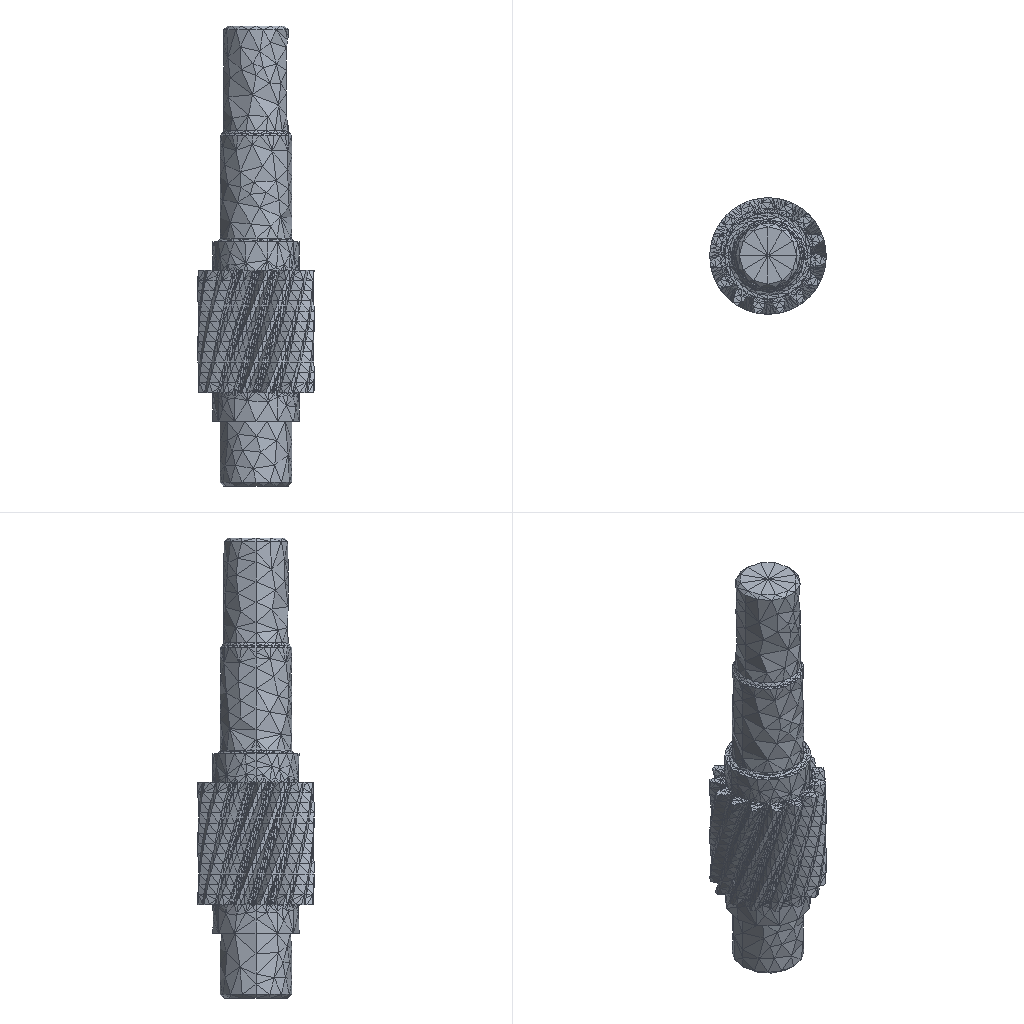Simulation study | ansys workbench
Ansys APDL input file, long lists of numbers shortened:
/batch
/config,noeldb,1     ! force off writing results to database
*get,_wallstrt,active,,time,wall
! ANSYS input file written by Workbench version 2022 R1
! File used for geometry attach: F:\ansys（分析文件汇总)\轴有限元分析\小斜齿轮优化.STEP
/title,wbnew--____ (D5)
! ****** Begin Custom Load Command Snippet ******
/COM, ACT Extensions:
/COM,     LSDYNA, 2021.1
/COM,
! ****** End   Custom Load Command Snippet ******
*DIM,_wb_ProjectScratch_dir,string,248
_wb_ProjectScratch_dir(1) = 'C:\Users\Administrator\AppData\Local\Temp\WB_Administrator_4372_2\_ProjectScratch\Scr3284\'
*DIM,_wb_SolverFiles_dir,string,248
_wb_SolverFiles_dir(1) = 'C:\Users\Administrator\AppData\Local\Temp\WB_Administrator_4372_2\wbnew_files\dp0\SYS-2\MECH\'
*DIM,_wb_userfiles_dir,string,248
_wb_userfiles_dir(1) = 'C:\Users\Administrator\AppData\Local\Temp\WB_Administrator_4372_2\wbnew_files\user_files\'
/com,--- Data in consistent NMM units. See Solving Units in the help system for more information.
/units,MPA
/nopr
/wb,file,start              !  signify a WB generated input file
/prep7
! Turn off shape checking because checks already performed inside WB mesher.
! See help system for more information.
SHPP,OFF,,NOWARN
/nolist
etcon,set             ! allow ANSYS to choose best KEYOP's for 180x elements, resets any applicable keyopt to MAPDL defaults
/com,*********** Nodes for the whole assembly ***********
nblock,3,,27687
(1i9,3e20.9e3)
        1     9.500000000E+00     3.266688912E-16     7.200000000E+01
! (25169 more lines like these left out)
-1
/com,*********** Nodes for all Remote Points ***********
nblock,3
(1i9,3e20.9e3)
    25171     1.031662461E+00     1.418091306E+00     3.522795447E+01
-1
/wb,elem,start            !  set before creation of elements
/com,*********** Elements for Body 1 "______-FreeParts|NONE" ***********
et,1,187
eblock,19,solid,,14648
(19i9)
        1        1        1        1        0        0        0        0       10        0        1     1980     1981     3907     3469    16186    16206    16197    16192
! (29295 more lines like these left out)
-1
/wb,elem,end               !  done creating elements
/com,*********** Send User Defined Coordinate System(s) ***********
csys,0
toffst,273.15,  ! Temperature offset from absolute zero
/com,*********** Set Reference Temperature ***********
tref,22.
/wb,mat,start              !  starting to send materials
/com,*********** Send Materials ***********
Temperature = 'TEMP' ! Temperature
MP,DENS,1,7.85e-09,	! tonne mm^-3
MP,ALPX,1,1.2e-05,	! C^-1
MP,C,1,434000000,	! mm^2 s^-2 C^-1
MP,KXX,1,60.5,	! tonne mm s^-3 C^-1
MP,RSVX,1,0.00017,	! ohm mm
MP,EX,1,200000,	! tonne s^-2 mm^-1
MP,NUXY,1,0.3,
MP,MURX,1,10000,
/wb,mat,end                !  done sending materials
!************************* Model Summary ********************
!______-FreeParts|NONE,	结构钢,	matid,	1
!************************* End Model Summary ********************
! get the diagonal of the bounding box. Needed later for other things
*get,_xmin,node,,mnloc,x
*get,_ymin,node,,mnloc,y
*get,_zmin,node,,mnloc,z
*get,_xmax,node,,mxloc,x
*get,_ymax,node,,mxloc,y
*get,_zmax,node,,mxloc,z
_ASMDIAG=(_xmax-_xmin)*(_xmax-_xmin)+(_ymax-_ymin)*(_ymax-_ymin)+(_zmax-_zmin)*(_zmax-_zmin)
_ASMDIAG=SQRT(_ASMDIAG)
/wb,contact,start          !  starting to send contact
/wb,contact,end            !  done creating contacts
/golist
/wb,load,start             !  starting to send loads
/com,*********** Fixed Supports ***********
CMBLOCK,_FIXEDSU,NODE,      513
(8i10)
        46        47        48        49        50        51        52        53
! (64 more lines like these left out)
cmsel,s,_FIXEDSU
d,all,all
nsel,all
/com,*********** Create Remote Point "内部远程点" ***********
! -------- Remote Point Used by "力矩" --------
*set,tid,3
*set,cid,2
et,cid,174
et,tid,170
keyo,tid,2,1               ! Don't fix the pilot node
keyo,tid,4,111111
keyo,cid,12,5              ! Bonded Contact
keyo,cid,4,1               ! Deformable RBE3 style load
keyo,cid,2,2               ! MPC style contact
eblock,10,,,605
(15i9)
    20068        2        2        2        0       79     1015     1879     1879     4359    11260     1879     4361
! (604 more lines like these left out)
-1
*set,_npilot,25171
_npilot32=_npilot
type,tid
mat ,cid
real,cid
tshape,pilo
en,20673,_npilot
tshape
/com,*********** Construct Moment Using Remote Attachment ***********
/gst,on,on
fini
*get,_numnode,node,0,count
*get,_numelem,elem,0,count
*get, _MAXELEMNUM, elem, 0, NUM, MAX
*get, _MAXNODENUM, node, 0, NUM, MAX
*get, _MAXELEMTYPE, etyp, 0, NUM, MAX
*get, _MAXREALCONST, real, 0, NUM, MAX
/go
/wb,load,end               !  done creating loads
/com,--- Number of total nodes = %_numnode%
/com,--- Number of contact elements = 605
/com,--- Number of spring elements = 0
/com,--- Number of bearing elements = 0
/com,--- Number of solid elements = 14648
/com,--- Number of condensed parts = 0
/com,--- Number of total elements = %_numelem%
*get,_wallbsol,active,,time,wall
/com,****************************************************************************
/com,*************************    SOLUTION       ********************************
/com,****************************************************************************
/solu
antype,0                   ! static analysis
_thickRatio=  1     ! Ratio of thick parts in the model
eqsl,pcg,1e-8,,,,,,1
cntr,print,1               ! print out contact info and also make no initial contact an error
dmpoption,emat,no             ! Don't combine emat file for DANSYS
dmpoption,esav,no             ! Don't combine esav file for DANSYS
nldiag,cont,iter           ! print out contact info each equilibrium iteration
rescontrol,,none                 ! Do not keep any restart files
/com,****************************************************
/com,******************* SOLVE FOR LS 1 OF 1 ****************
nsel,s,node,,25171
f,all,mx,0.
f,all,my,500000.
f,all,mz,0.
nsel,all
/nopr
/gopr
nsub,1,1,1
time,1.
outres,erase
outres,all,none
outres,nsol,all,
outres,rsol,all
outres,eangl,all
outres,etmp,all
outres,veng,all
outres,strs,all,
outres,epel,all,
outres,eppl,all,
outres,cont,all,
! *********** WB SOLVE COMMAND ***********
! check interactive state
*get,ANSINTER_,active,,int
*if,ANSINTER_,ne,0,then
/eof
*endif
solve
/com *************** Write FE CONNECTORS *********
CEWRITE,file,ce,,INTE
/com,****************************************************
/com,*************** FINISHED SOLVE FOR LS 1 *************
*get,_wallasol,active,,time,wall
/nopr
*get,_numnode,node,0,count
*get,_numelem,elem,0,count
*get, _MAXELEMNUM, elem, 0, NUM, MAX
*get, _MAXNODENUM, node, 0, NUM, MAX,,,INTERNAL
*get, _MAXELEMTYPE, etyp, 0, NUM, MAX
*get, _MAXREALCONST, real, 0, NUM, MAX
/gopr
*get,_PCGITER,active,,solu,cgiter
/post1
xmlo,ENCODING,ISO-8859-1
xmlo,parm
/xml,parm,xml
fini
/gopr
*get,_walldone,active,,time,wall
_preptime=(_wallbsol-_wallstrt)*3600
_solvtime=(_wallasol-_wallbsol)*3600
_posttime=(_walldone-_wallasol)*3600
_totaltim=(_walldone-_wallstrt)*3600
*get,_dlbratio,active,0,solu,dlbr
*get,_combtime,active,0,solu,comb
*get,_ssmode,active,0,solu,ssmm
*get,_ndofs,active,0,solu,ndof
*get,_sol_end_time,active,0,set,time
*if,_sol_end_time,eq,1.,then
/fclean				!clean distributed files
*endif
/com,--- Total number of nodes = %_numnode%
/com,--- Total number of elements = %_numelem%
/com,--- Element load balance ratio = %_dlbratio%
/com,--- Time to combine distributed files = %_combtime%
/com,--- Sparse memory mode = %_ssmode%
/com,--- Number of DOF = %_ndofs%
/wb,file,end               ! done with WB generated input